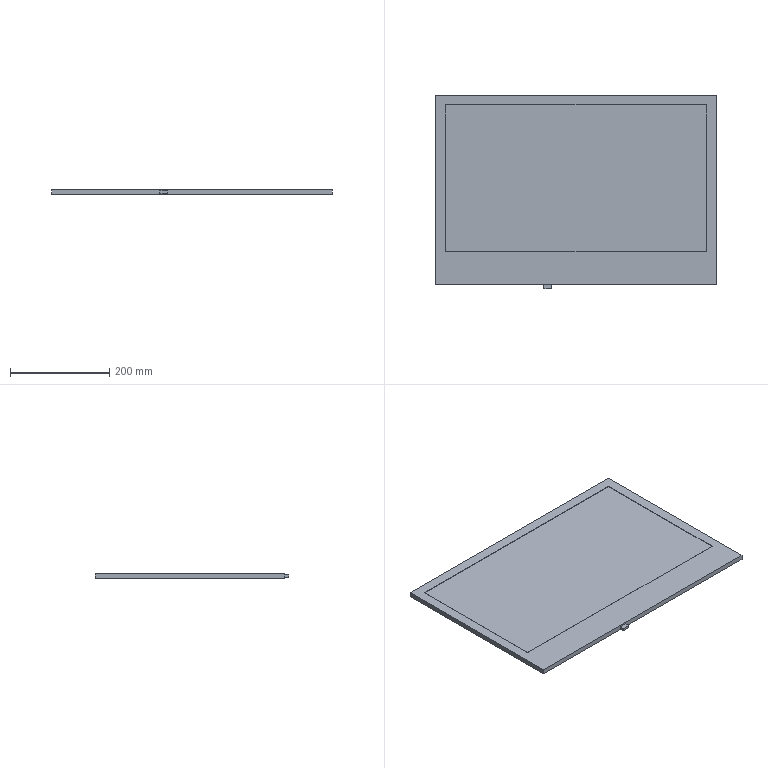Part | STEP file | 23.6 inch screen 01001 | 2 solids | 22 faces | box 564 x 390 x 10 mm | volume 1834790 mm3 | plane 22
STEP:
#1=CARTESIAN_POINT('',(0.,0.,0.));
#2=DIRECTION('',(0.,0.,1.));
#3=DIRECTION('',(1.,0.,0.));
#4=AXIS2_PLACEMENT_3D('',#1,#2,#3);
#5=CARTESIAN_POINT('',(282.,-190.,-5.));
#6=VERTEX_POINT('',#5);
#7=CARTESIAN_POINT('',(282.,190.,-5.));
#8=VERTEX_POINT('',#7);
#9=CARTESIAN_POINT('',(282.,-190.,-5.));
#10=DIRECTION('',(0.,1.,0.));
#11=VECTOR('',#10,1.);
#12=LINE('',#9,#11);
#13=CARTESIAN_POINT('',(0.,0.,-5.));
#14=DIRECTION('',(0.,0.,-1.));
#15=DIRECTION('',(-1.,0.,0.));
#16=AXIS2_PLACEMENT_3D('',#13,#14,#15);
#17=PLANE('',#16);
#18=CARTESIAN_POINT('',(-282.,-190.));
#19=DIRECTION('',(0.,1.));
#20=VECTOR('',#19,1.);
#21=LINE('',#18,#20);
#22=(GEOMETRIC_REPRESENTATION_CONTEXT(2)PARAMETRIC_REPRESENTATION_CONTEXT()REPRESENTATION_CONTEXT('',''));
#23=DEFINITIONAL_REPRESENTATION('',(#21),#22);
#24=PCURVE('',#17,#23);
#25=CARTESIAN_POINT('',(282.,-190.,5.));
#26=DIRECTION('',(-1.,0.,0.));
#27=DIRECTION('',(0.,0.,1.));
#28=AXIS2_PLACEMENT_3D('',#25,#26,#27);
#29=PLANE('',#28);
#30=CARTESIAN_POINT('',(-10.,0.));
#31=DIRECTION('',(0.,1.));
#32=VECTOR('',#31,1.);
#33=LINE('',#30,#32);
#34=(GEOMETRIC_REPRESENTATION_CONTEXT(2)PARAMETRIC_REPRESENTATION_CONTEXT()REPRESENTATION_CONTEXT('',''));
#35=DEFINITIONAL_REPRESENTATION('',(#33),#34);
#36=PCURVE('',#29,#35);
#37=SURFACE_CURVE('',#12,(#24,#36),.PCURVE_S1.);
#38=EDGE_CURVE('',#6,#8,#37,.T.);
#39=ORIENTED_EDGE('',*,*,#38,.F.);
#40=CARTESIAN_POINT('',(-282.,-190.,-5.));
#41=VERTEX_POINT('',#40);
#42=CARTESIAN_POINT('',(-282.,-190.,-5.));
#43=DIRECTION('',(1.,0.,0.));
#44=VECTOR('',#43,1.);
#45=LINE('',#42,#44);
#46=CARTESIAN_POINT('',(282.,-190.));
#47=DIRECTION('',(-1.,0.));
#48=VECTOR('',#47,1.);
#49=LINE('',#46,#48);
#50=(GEOMETRIC_REPRESENTATION_CONTEXT(2)PARAMETRIC_REPRESENTATION_CONTEXT()REPRESENTATION_CONTEXT('',''));
#51=DEFINITIONAL_REPRESENTATION('',(#49),#50);
#52=PCURVE('',#17,#51);
#53=CARTESIAN_POINT('',(-282.,-190.,5.));
#54=DIRECTION('',(0.,1.,0.));
#55=DIRECTION('',(0.,0.,1.));
#56=AXIS2_PLACEMENT_3D('',#53,#54,#55);
#57=PLANE('',#56);
#58=CARTESIAN_POINT('',(-10.,0.));
#59=DIRECTION('',(0.,1.));
#60=VECTOR('',#59,1.);
#61=LINE('',#58,#60);
#62=(GEOMETRIC_REPRESENTATION_CONTEXT(2)PARAMETRIC_REPRESENTATION_CONTEXT()REPRESENTATION_CONTEXT('',''));
#63=DEFINITIONAL_REPRESENTATION('',(#61),#62);
#64=PCURVE('',#57,#63);
#65=SURFACE_CURVE('',#45,(#52,#64),.PCURVE_S1.);
#66=EDGE_CURVE('',#41,#6,#65,.T.);
#67=ORIENTED_EDGE('',*,*,#66,.F.);
#68=CARTESIAN_POINT('',(-282.,190.,-5.));
#69=VERTEX_POINT('',#68);
#70=CARTESIAN_POINT('',(-282.,-190.,-5.));
#71=DIRECTION('',(0.,-1.,0.));
#72=VECTOR('',#71,1.);
#73=LINE('',#70,#72);
#74=CARTESIAN_POINT('',(282.,-190.));
#75=DIRECTION('',(0.,-1.));
#76=VECTOR('',#75,1.);
#77=LINE('',#74,#76);
#78=(GEOMETRIC_REPRESENTATION_CONTEXT(2)PARAMETRIC_REPRESENTATION_CONTEXT()REPRESENTATION_CONTEXT('',''));
#79=DEFINITIONAL_REPRESENTATION('',(#77),#78);
#80=PCURVE('',#17,#79);
#81=CARTESIAN_POINT('',(-282.,-190.,5.));
#82=DIRECTION('',(1.,0.,0.));
#83=DIRECTION('',(0.,0.,-1.));
#84=AXIS2_PLACEMENT_3D('',#81,#82,#83);
#85=PLANE('',#84);
#86=CARTESIAN_POINT('',(10.,0.));
#87=DIRECTION('',(0.,-1.));
#88=VECTOR('',#87,1.);
#89=LINE('',#86,#88);
#90=(GEOMETRIC_REPRESENTATION_CONTEXT(2)PARAMETRIC_REPRESENTATION_CONTEXT()REPRESENTATION_CONTEXT('',''));
#91=DEFINITIONAL_REPRESENTATION('',(#89),#90);
#92=PCURVE('',#85,#91);
#93=SURFACE_CURVE('',#73,(#80,#92),.PCURVE_S1.);
#94=EDGE_CURVE('',#69,#41,#93,.T.);
#95=ORIENTED_EDGE('',*,*,#94,.F.);
#96=CARTESIAN_POINT('',(-282.,190.,-5.));
#97=DIRECTION('',(-1.,0.,0.));
#98=VECTOR('',#97,1.);
#99=LINE('',#96,#98);
#100=CARTESIAN_POINT('',(282.,190.));
#101=DIRECTION('',(1.,0.));
#102=VECTOR('',#101,1.);
#103=LINE('',#100,#102);
#104=(GEOMETRIC_REPRESENTATION_CONTEXT(2)PARAMETRIC_REPRESENTATION_CONTEXT()REPRESENTATION_CONTEXT('',''));
#105=DEFINITIONAL_REPRESENTATION('',(#103),#104);
#106=PCURVE('',#17,#105);
#107=CARTESIAN_POINT('',(-282.,190.,5.));
#108=DIRECTION('',(0.,-1.,0.));
#109=DIRECTION('',(0.,0.,-1.));
#110=AXIS2_PLACEMENT_3D('',#107,#108,#109);
#111=PLANE('',#110);
#112=CARTESIAN_POINT('',(10.,0.));
#113=DIRECTION('',(0.,-1.));
#114=VECTOR('',#113,1.);
#115=LINE('',#112,#114);
#116=(GEOMETRIC_REPRESENTATION_CONTEXT(2)PARAMETRIC_REPRESENTATION_CONTEXT()REPRESENTATION_CONTEXT('',''));
#117=DEFINITIONAL_REPRESENTATION('',(#115),#116);
#118=PCURVE('',#111,#117);
#119=SURFACE_CURVE('',#99,(#106,#118),.PCURVE_S1.);
#120=EDGE_CURVE('',#8,#69,#119,.T.);
#121=ORIENTED_EDGE('',*,*,#120,.F.);
#122=EDGE_LOOP('',(#39,#67,#95,#121));
#123=FACE_BOUND('',#122,.T.);
#124=CARTESIAN_POINT('',(-262.,-125.,-5.));
#125=VERTEX_POINT('',#124);
#126=CARTESIAN_POINT('',(262.,-125.,-5.));
#127=VERTEX_POINT('',#126);
#128=CARTESIAN_POINT('',(-262.,-125.,-5.));
#129=DIRECTION('',(1.,0.,0.));
#130=VECTOR('',#129,1.);
#131=LINE('',#128,#130);
#132=CARTESIAN_POINT('',(262.,-125.));
#133=DIRECTION('',(-1.,0.));
#134=VECTOR('',#133,1.);
#135=LINE('',#132,#134);
#136=(GEOMETRIC_REPRESENTATION_CONTEXT(2)PARAMETRIC_REPRESENTATION_CONTEXT()REPRESENTATION_CONTEXT('',''));
#137=DEFINITIONAL_REPRESENTATION('',(#135),#136);
#138=PCURVE('',#17,#137);
#139=CARTESIAN_POINT('',(-262.,-125.,-4.));
#140=DIRECTION('',(0.,1.,0.));
#141=DIRECTION('',(0.,0.,1.));
#142=AXIS2_PLACEMENT_3D('',#139,#140,#141);
#143=PLANE('',#142);
#144=CARTESIAN_POINT('',(-1.,0.));
#145=DIRECTION('',(0.,1.));
#146=VECTOR('',#145,1.);
#147=LINE('',#144,#146);
#148=(GEOMETRIC_REPRESENTATION_CONTEXT(2)PARAMETRIC_REPRESENTATION_CONTEXT()REPRESENTATION_CONTEXT('',''));
#149=DEFINITIONAL_REPRESENTATION('',(#147),#148);
#150=PCURVE('',#143,#149);
#151=SURFACE_CURVE('',#131,(#138,#150),.PCURVE_S1.);
#152=EDGE_CURVE('',#125,#127,#151,.T.);
#153=ORIENTED_EDGE('',*,*,#152,.T.);
#154=CARTESIAN_POINT('',(262.,170.,-5.));
#155=VERTEX_POINT('',#154);
#156=CARTESIAN_POINT('',(262.,-125.,-5.));
#157=DIRECTION('',(0.,1.,0.));
#158=VECTOR('',#157,1.);
#159=LINE('',#156,#158);
#160=CARTESIAN_POINT('',(-262.,-125.));
#161=DIRECTION('',(0.,1.));
#162=VECTOR('',#161,1.);
#163=LINE('',#160,#162);
#164=(GEOMETRIC_REPRESENTATION_CONTEXT(2)PARAMETRIC_REPRESENTATION_CONTEXT()REPRESENTATION_CONTEXT('',''));
#165=DEFINITIONAL_REPRESENTATION('',(#163),#164);
#166=PCURVE('',#17,#165);
#167=CARTESIAN_POINT('',(262.,-125.,-4.));
#168=DIRECTION('',(-1.,0.,0.));
#169=DIRECTION('',(0.,0.,1.));
#170=AXIS2_PLACEMENT_3D('',#167,#168,#169);
#171=PLANE('',#170);
#172=CARTESIAN_POINT('',(-1.,0.));
#173=DIRECTION('',(0.,1.));
#174=VECTOR('',#173,1.);
#175=LINE('',#172,#174);
#176=(GEOMETRIC_REPRESENTATION_CONTEXT(2)PARAMETRIC_REPRESENTATION_CONTEXT()REPRESENTATION_CONTEXT('',''));
#177=DEFINITIONAL_REPRESENTATION('',(#175),#176);
#178=PCURVE('',#171,#177);
#179=SURFACE_CURVE('',#159,(#166,#178),.PCURVE_S1.);
#180=EDGE_CURVE('',#127,#155,#179,.T.);
#181=ORIENTED_EDGE('',*,*,#180,.T.);
#182=CARTESIAN_POINT('',(-262.,170.,-5.));
#183=VERTEX_POINT('',#182);
#184=CARTESIAN_POINT('',(-262.,170.,-5.));
#185=DIRECTION('',(-1.,0.,0.));
#186=VECTOR('',#185,1.);
#187=LINE('',#184,#186);
#188=CARTESIAN_POINT('',(262.,170.));
#189=DIRECTION('',(1.,0.));
#190=VECTOR('',#189,1.);
#191=LINE('',#188,#190);
#192=(GEOMETRIC_REPRESENTATION_CONTEXT(2)PARAMETRIC_REPRESENTATION_CONTEXT()REPRESENTATION_CONTEXT('',''));
#193=DEFINITIONAL_REPRESENTATION('',(#191),#192);
#194=PCURVE('',#17,#193);
#195=CARTESIAN_POINT('',(-262.,170.,-4.));
#196=DIRECTION('',(0.,-1.,0.));
#197=DIRECTION('',(0.,0.,-1.));
#198=AXIS2_PLACEMENT_3D('',#195,#196,#197);
#199=PLANE('',#198);
#200=CARTESIAN_POINT('',(1.,0.));
#201=DIRECTION('',(0.,-1.));
#202=VECTOR('',#201,1.);
#203=LINE('',#200,#202);
#204=(GEOMETRIC_REPRESENTATION_CONTEXT(2)PARAMETRIC_REPRESENTATION_CONTEXT()REPRESENTATION_CONTEXT('',''));
#205=DEFINITIONAL_REPRESENTATION('',(#203),#204);
#206=PCURVE('',#199,#205);
#207=SURFACE_CURVE('',#187,(#194,#206),.PCURVE_S1.);
#208=EDGE_CURVE('',#155,#183,#207,.T.);
#209=ORIENTED_EDGE('',*,*,#208,.T.);
#210=CARTESIAN_POINT('',(-262.,-125.,-5.));
#211=DIRECTION('',(0.,-1.,0.));
#212=VECTOR('',#211,1.);
#213=LINE('',#210,#212);
#214=CARTESIAN_POINT('',(262.,-125.));
#215=DIRECTION('',(0.,-1.));
#216=VECTOR('',#215,1.);
#217=LINE('',#214,#216);
#218=(GEOMETRIC_REPRESENTATION_CONTEXT(2)PARAMETRIC_REPRESENTATION_CONTEXT()REPRESENTATION_CONTEXT('',''));
#219=DEFINITIONAL_REPRESENTATION('',(#217),#218);
#220=PCURVE('',#17,#219);
#221=CARTESIAN_POINT('',(-262.,-125.,-4.));
#222=DIRECTION('',(1.,0.,0.));
#223=DIRECTION('',(0.,0.,-1.));
#224=AXIS2_PLACEMENT_3D('',#221,#222,#223);
#225=PLANE('',#224);
#226=CARTESIAN_POINT('',(1.,0.));
#227=DIRECTION('',(0.,-1.));
#228=VECTOR('',#227,1.);
#229=LINE('',#226,#228);
#230=(GEOMETRIC_REPRESENTATION_CONTEXT(2)PARAMETRIC_REPRESENTATION_CONTEXT()REPRESENTATION_CONTEXT('',''));
#231=DEFINITIONAL_REPRESENTATION('',(#229),#230);
#232=PCURVE('',#225,#231);
#233=SURFACE_CURVE('',#213,(#220,#232),.PCURVE_S1.);
#234=EDGE_CURVE('',#183,#125,#233,.T.);
#235=ORIENTED_EDGE('',*,*,#234,.T.);
#236=EDGE_LOOP('',(#153,#181,#209,#235));
#237=FACE_BOUND('',#236,.T.);
#238=ADVANCED_FACE('',(#123,#237),#17,.T.);
#239=ORIENTED_EDGE('',*,*,#38,.T.);
#240=CARTESIAN_POINT('',(282.,190.,5.));
#241=VERTEX_POINT('',#240);
#242=CARTESIAN_POINT('',(282.,190.,5.));
#243=DIRECTION('',(0.,0.,-1.));
#244=VECTOR('',#243,1.);
#245=LINE('',#242,#244);
#246=CARTESIAN_POINT('',(0.,380.));
#247=DIRECTION('',(-1.,0.));
#248=VECTOR('',#247,1.);
#249=LINE('',#246,#248);
#250=(GEOMETRIC_REPRESENTATION_CONTEXT(2)PARAMETRIC_REPRESENTATION_CONTEXT()REPRESENTATION_CONTEXT('',''));
#251=DEFINITIONAL_REPRESENTATION('',(#249),#250);
#252=PCURVE('',#29,#251);
#253=CARTESIAN_POINT('',(0.,564.));
#254=DIRECTION('',(1.,0.));
#255=VECTOR('',#254,1.);
#256=LINE('',#253,#255);
#257=(GEOMETRIC_REPRESENTATION_CONTEXT(2)PARAMETRIC_REPRESENTATION_CONTEXT()REPRESENTATION_CONTEXT('',''));
#258=DEFINITIONAL_REPRESENTATION('',(#256),#257);
#259=PCURVE('',#111,#258);
#260=SURFACE_CURVE('',#245,(#252,#259),.PCURVE_S1.);
#261=EDGE_CURVE('',#241,#8,#260,.T.);
#262=ORIENTED_EDGE('',*,*,#261,.F.);
#263=CARTESIAN_POINT('',(282.,-190.,5.));
#264=VERTEX_POINT('',#263);
#265=CARTESIAN_POINT('',(282.,-190.,5.));
#266=DIRECTION('',(0.,1.,0.));
#267=VECTOR('',#266,1.);
#268=LINE('',#265,#267);
#269=CARTESIAN_POINT('',(0.,0.));
#270=DIRECTION('',(0.,1.));
#271=VECTOR('',#270,1.);
#272=LINE('',#269,#271);
#273=(GEOMETRIC_REPRESENTATION_CONTEXT(2)PARAMETRIC_REPRESENTATION_CONTEXT()REPRESENTATION_CONTEXT('',''));
#274=DEFINITIONAL_REPRESENTATION('',(#272),#273);
#275=PCURVE('',#29,#274);
#276=CARTESIAN_POINT('',(0.,0.,5.));
#277=DIRECTION('',(0.,0.,-1.));
#278=DIRECTION('',(-1.,0.,0.));
#279=AXIS2_PLACEMENT_3D('',#276,#277,#278);
#280=PLANE('',#279);
#281=CARTESIAN_POINT('',(-282.,-190.));
#282=DIRECTION('',(0.,1.));
#283=VECTOR('',#282,1.);
#284=LINE('',#281,#283);
#285=(GEOMETRIC_REPRESENTATION_CONTEXT(2)PARAMETRIC_REPRESENTATION_CONTEXT()REPRESENTATION_CONTEXT('',''));
#286=DEFINITIONAL_REPRESENTATION('',(#284),#285);
#287=PCURVE('',#280,#286);
#288=SURFACE_CURVE('',#268,(#275,#287),.PCURVE_S1.);
#289=EDGE_CURVE('',#264,#241,#288,.T.);
#290=ORIENTED_EDGE('',*,*,#289,.F.);
#291=CARTESIAN_POINT('',(282.,-190.,5.));
#292=DIRECTION('',(0.,0.,-1.));
#293=VECTOR('',#292,1.);
#294=LINE('',#291,#293);
#295=CARTESIAN_POINT('',(0.,0.));
#296=DIRECTION('',(-1.,0.));
#297=VECTOR('',#296,1.);
#298=LINE('',#295,#297);
#299=(GEOMETRIC_REPRESENTATION_CONTEXT(2)PARAMETRIC_REPRESENTATION_CONTEXT()REPRESENTATION_CONTEXT('',''));
#300=DEFINITIONAL_REPRESENTATION('',(#298),#299);
#301=PCURVE('',#29,#300);
#302=CARTESIAN_POINT('',(0.,564.));
#303=DIRECTION('',(-1.,0.));
#304=VECTOR('',#303,1.);
#305=LINE('',#302,#304);
#306=(GEOMETRIC_REPRESENTATION_CONTEXT(2)PARAMETRIC_REPRESENTATION_CONTEXT()REPRESENTATION_CONTEXT('',''));
#307=DEFINITIONAL_REPRESENTATION('',(#305),#306);
#308=PCURVE('',#57,#307);
#309=SURFACE_CURVE('',#294,(#301,#308),.PCURVE_S1.);
#310=EDGE_CURVE('',#264,#6,#309,.T.);
#311=ORIENTED_EDGE('',*,*,#310,.T.);
#312=EDGE_LOOP('',(#239,#262,#290,#311));
#313=FACE_BOUND('',#312,.T.);
#314=ADVANCED_FACE('',(#313),#29,.F.);
#315=ORIENTED_EDGE('',*,*,#120,.T.);
#316=CARTESIAN_POINT('',(-282.,190.,5.));
#317=VERTEX_POINT('',#316);
#318=CARTESIAN_POINT('',(-282.,190.,5.));
#319=DIRECTION('',(0.,0.,-1.));
#320=VECTOR('',#319,1.);
#321=LINE('',#318,#320);
#322=CARTESIAN_POINT('',(0.,0.));
#323=DIRECTION('',(1.,0.));
#324=VECTOR('',#323,1.);
#325=LINE('',#322,#324);
#326=(GEOMETRIC_REPRESENTATION_CONTEXT(2)PARAMETRIC_REPRESENTATION_CONTEXT()REPRESENTATION_CONTEXT('',''));
#327=DEFINITIONAL_REPRESENTATION('',(#325),#326);
#328=PCURVE('',#111,#327);
#329=CARTESIAN_POINT('',(0.,380.));
#330=DIRECTION('',(1.,0.));
#331=VECTOR('',#330,1.);
#332=LINE('',#329,#331);
#333=(GEOMETRIC_REPRESENTATION_CONTEXT(2)PARAMETRIC_REPRESENTATION_CONTEXT()REPRESENTATION_CONTEXT('',''));
#334=DEFINITIONAL_REPRESENTATION('',(#332),#333);
#335=PCURVE('',#85,#334);
#336=SURFACE_CURVE('',#321,(#328,#335),.PCURVE_S1.);
#337=EDGE_CURVE('',#317,#69,#336,.T.);
#338=ORIENTED_EDGE('',*,*,#337,.F.);
#339=CARTESIAN_POINT('',(-282.,190.,5.));
#340=DIRECTION('',(-1.,0.,0.));
#341=VECTOR('',#340,1.);
#342=LINE('',#339,#341);
#343=CARTESIAN_POINT('',(0.,0.));
#344=DIRECTION('',(0.,-1.));
#345=VECTOR('',#344,1.);
#346=LINE('',#343,#345);
#347=(GEOMETRIC_REPRESENTATION_CONTEXT(2)PARAMETRIC_REPRESENTATION_CONTEXT()REPRESENTATION_CONTEXT('',''));
#348=DEFINITIONAL_REPRESENTATION('',(#346),#347);
#349=PCURVE('',#111,#348);
#350=CARTESIAN_POINT('',(282.,190.));
#351=DIRECTION('',(1.,0.));
#352=VECTOR('',#351,1.);
#353=LINE('',#350,#352);
#354=(GEOMETRIC_REPRESENTATION_CONTEXT(2)PARAMETRIC_REPRESENTATION_CONTEXT()REPRESENTATION_CONTEXT('',''));
#355=DEFINITIONAL_REPRESENTATION('',(#353),#354);
#356=PCURVE('',#280,#355);
#357=SURFACE_CURVE('',#342,(#349,#356),.PCURVE_S1.);
#358=EDGE_CURVE('',#241,#317,#357,.T.);
#359=ORIENTED_EDGE('',*,*,#358,.F.);
#360=ORIENTED_EDGE('',*,*,#261,.T.);
#361=EDGE_LOOP('',(#315,#338,#359,#360));
#362=FACE_BOUND('',#361,.T.);
#363=ADVANCED_FACE('',(#362),#111,.F.);
#364=ORIENTED_EDGE('',*,*,#94,.T.);
#365=CARTESIAN_POINT('',(-282.,-190.,5.));
#366=VERTEX_POINT('',#365);
#367=CARTESIAN_POINT('',(-282.,-190.,5.));
#368=DIRECTION('',(0.,0.,-1.));
#369=VECTOR('',#368,1.);
#370=LINE('',#367,#369);
#371=CARTESIAN_POINT('',(0.,0.));
#372=DIRECTION('',(1.,0.));
#373=VECTOR('',#372,1.);
#374=LINE('',#371,#373);
#375=(GEOMETRIC_REPRESENTATION_CONTEXT(2)PARAMETRIC_REPRESENTATION_CONTEXT()REPRESENTATION_CONTEXT('',''));
#376=DEFINITIONAL_REPRESENTATION('',(#374),#375);
#377=PCURVE('',#85,#376);
#378=CARTESIAN_POINT('',(0.,0.));
#379=DIRECTION('',(-1.,0.));
#380=VECTOR('',#379,1.);
#381=LINE('',#378,#380);
#382=(GEOMETRIC_REPRESENTATION_CONTEXT(2)PARAMETRIC_REPRESENTATION_CONTEXT()REPRESENTATION_CONTEXT('',''));
#383=DEFINITIONAL_REPRESENTATION('',(#381),#382);
#384=PCURVE('',#57,#383);
#385=SURFACE_CURVE('',#370,(#377,#384),.PCURVE_S1.);
#386=EDGE_CURVE('',#366,#41,#385,.T.);
#387=ORIENTED_EDGE('',*,*,#386,.F.);
#388=CARTESIAN_POINT('',(-282.,-190.,5.));
#389=DIRECTION('',(0.,-1.,0.));
#390=VECTOR('',#389,1.);
#391=LINE('',#388,#390);
#392=CARTESIAN_POINT('',(0.,0.));
#393=DIRECTION('',(0.,-1.));
#394=VECTOR('',#393,1.);
#395=LINE('',#392,#394);
#396=(GEOMETRIC_REPRESENTATION_CONTEXT(2)PARAMETRIC_REPRESENTATION_CONTEXT()REPRESENTATION_CONTEXT('',''));
#397=DEFINITIONAL_REPRESENTATION('',(#395),#396);
#398=PCURVE('',#85,#397);
#399=CARTESIAN_POINT('',(282.,-190.));
#400=DIRECTION('',(0.,-1.));
#401=VECTOR('',#400,1.);
#402=LINE('',#399,#401);
#403=(GEOMETRIC_REPRESENTATION_CONTEXT(2)PARAMETRIC_REPRESENTATION_CONTEXT()REPRESENTATION_CONTEXT('',''));
#404=DEFINITIONAL_REPRESENTATION('',(#402),#403);
#405=PCURVE('',#280,#404);
#406=SURFACE_CURVE('',#391,(#398,#405),.PCURVE_S1.);
#407=EDGE_CURVE('',#317,#366,#406,.T.);
#408=ORIENTED_EDGE('',*,*,#407,.F.);
#409=ORIENTED_EDGE('',*,*,#337,.T.);
#410=EDGE_LOOP('',(#364,#387,#408,#409));
#411=FACE_BOUND('',#410,.T.);
#412=ADVANCED_FACE('',(#411),#85,.F.);
#413=ORIENTED_EDGE('',*,*,#66,.T.);
#414=ORIENTED_EDGE('',*,*,#310,.F.);
#415=CARTESIAN_POINT('',(-282.,-190.,5.));
#416=DIRECTION('',(1.,0.,0.));
#417=VECTOR('',#416,1.);
#418=LINE('',#415,#417);
#419=CARTESIAN_POINT('',(0.,0.));
#420=DIRECTION('',(0.,1.));
#421=VECTOR('',#420,1.);
#422=LINE('',#419,#421);
#423=(GEOMETRIC_REPRESENTATION_CONTEXT(2)PARAMETRIC_REPRESENTATION_CONTEXT()REPRESENTATION_CONTEXT('',''));
#424=DEFINITIONAL_REPRESENTATION('',(#422),#423);
#425=PCURVE('',#57,#424);
#426=CARTESIAN_POINT('',(282.,-190.));
#427=DIRECTION('',(-1.,0.));
#428=VECTOR('',#427,1.);
#429=LINE('',#426,#428);
#430=(GEOMETRIC_REPRESENTATION_CONTEXT(2)PARAMETRIC_REPRESENTATION_CONTEXT()REPRESENTATION_CONTEXT('',''));
#431=DEFINITIONAL_REPRESENTATION('',(#429),#430);
#432=PCURVE('',#280,#431);
#433=SURFACE_CURVE('',#418,(#425,#432),.PCURVE_S1.);
#434=EDGE_CURVE('',#366,#264,#433,.T.);
#435=ORIENTED_EDGE('',*,*,#434,.F.);
#436=ORIENTED_EDGE('',*,*,#386,.T.);
#437=EDGE_LOOP('',(#413,#414,#435,#436));
#438=FACE_BOUND('',#437,.T.);
#439=ADVANCED_FACE('',(#438),#57,.F.);
#440=CARTESIAN_POINT('',(262.,170.,5.));
#441=VERTEX_POINT('',#440);
#442=CARTESIAN_POINT('',(-262.,170.,5.));
#443=VERTEX_POINT('',#442);
#444=CARTESIAN_POINT('',(-262.,170.,5.));
#445=DIRECTION('',(-1.,0.,0.));
#446=VECTOR('',#445,1.);
#447=LINE('',#444,#446);
#448=CARTESIAN_POINT('',(262.,170.));
#449=DIRECTION('',(1.,0.));
#450=VECTOR('',#449,1.);
#451=LINE('',#448,#450);
#452=(GEOMETRIC_REPRESENTATION_CONTEXT(2)PARAMETRIC_REPRESENTATION_CONTEXT()REPRESENTATION_CONTEXT('',''));
#453=DEFINITIONAL_REPRESENTATION('',(#451),#452);
#454=PCURVE('',#280,#453);
#455=CARTESIAN_POINT('',(-262.,170.,4.));
#456=DIRECTION('',(0.,1.,0.));
#457=DIRECTION('',(0.,0.,1.));
#458=AXIS2_PLACEMENT_3D('',#455,#456,#457);
#459=PLANE('',#458);
#460=CARTESIAN_POINT('',(1.,0.));
#461=DIRECTION('',(0.,-1.));
#462=VECTOR('',#461,1.);
#463=LINE('',#460,#462);
#464=(GEOMETRIC_REPRESENTATION_CONTEXT(2)PARAMETRIC_REPRESENTATION_CONTEXT()REPRESENTATION_CONTEXT('',''));
#465=DEFINITIONAL_REPRESENTATION('',(#463),#464);
#466=PCURVE('',#459,#465);
#467=SURFACE_CURVE('',#447,(#454,#466),.PCURVE_S1.);
#468=EDGE_CURVE('',#441,#443,#467,.T.);
#469=ORIENTED_EDGE('',*,*,#468,.F.);
#470=CARTESIAN_POINT('',(262.,-125.,5.));
#471=VERTEX_POINT('',#470);
#472=CARTESIAN_POINT('',(262.,-125.,5.));
#473=DIRECTION('',(0.,1.,0.));
#474=VECTOR('',#473,1.);
#475=LINE('',#472,#474);
#476=CARTESIAN_POINT('',(-262.,-125.));
#477=DIRECTION('',(0.,1.));
#478=VECTOR('',#477,1.);
#479=LINE('',#476,#478);
#480=(GEOMETRIC_REPRESENTATION_CONTEXT(2)PARAMETRIC_REPRESENTATION_CONTEXT()REPRESENTATION_CONTEXT('',''));
#481=DEFINITIONAL_REPRESENTATION('',(#479),#480);
#482=PCURVE('',#280,#481);
#483=CARTESIAN_POINT('',(262.,-125.,4.));
#484=DIRECTION('',(1.,0.,0.));
#485=DIRECTION('',(0.,0.,-1.));
#486=AXIS2_PLACEMENT_3D('',#483,#484,#485);
#487=PLANE('',#486);
#488=CARTESIAN_POINT('',(-1.,0.));
#489=DIRECTION('',(0.,1.));
#490=VECTOR('',#489,1.);
#491=LINE('',#488,#490);
#492=(GEOMETRIC_REPRESENTATION_CONTEXT(2)PARAMETRIC_REPRESENTATION_CONTEXT()REPRESENTATION_CONTEXT('',''));
#493=DEFINITIONAL_REPRESENTATION('',(#491),#492);
#494=PCURVE('',#487,#493);
#495=SURFACE_CURVE('',#475,(#482,#494),.PCURVE_S1.);
#496=EDGE_CURVE('',#471,#441,#495,.T.);
#497=ORIENTED_EDGE('',*,*,#496,.F.);
#498=CARTESIAN_POINT('',(-262.,-125.,5.));
#499=VERTEX_POINT('',#498);
#500=CARTESIAN_POINT('',(-262.,-125.,5.));
#501=DIRECTION('',(1.,0.,0.));
#502=VECTOR('',#501,1.);
#503=LINE('',#500,#502);
#504=CARTESIAN_POINT('',(262.,-125.));
#505=DIRECTION('',(-1.,0.));
#506=VECTOR('',#505,1.);
#507=LINE('',#504,#506);
#508=(GEOMETRIC_REPRESENTATION_CONTEXT(2)PARAMETRIC_REPRESENTATION_CONTEXT()REPRESENTATION_CONTEXT('',''));
#509=DEFINITIONAL_REPRESENTATION('',(#507),#508);
#510=PCURVE('',#280,#509);
#511=CARTESIAN_POINT('',(-262.,-125.,4.));
#512=DIRECTION('',(0.,-1.,0.));
#513=DIRECTION('',(0.,0.,-1.));
#514=AXIS2_PLACEMENT_3D('',#511,#512,#513);
#515=PLANE('',#514);
#516=CARTESIAN_POINT('',(-1.,0.));
#517=DIRECTION('',(0.,1.));
#518=VECTOR('',#517,1.);
#519=LINE('',#516,#518);
#520=(GEOMETRIC_REPRESENTATION_CONTEXT(2)PARAMETRIC_REPRESENTATION_CONTEXT()REPRESENTATION_CONTEXT('',''));
#521=DEFINITIONAL_REPRESENTATION('',(#519),#520);
#522=PCURVE('',#515,#521);
#523=SURFACE_CURVE('',#503,(#510,#522),.PCURVE_S1.);
#524=EDGE_CURVE('',#499,#471,#523,.T.);
#525=ORIENTED_EDGE('',*,*,#524,.F.);
#526=CARTESIAN_POINT('',(-262.,-125.,5.));
#527=DIRECTION('',(0.,-1.,0.));
#528=VECTOR('',#527,1.);
#529=LINE('',#526,#528);
#530=CARTESIAN_POINT('',(262.,-125.));
#531=DIRECTION('',(0.,-1.));
#532=VECTOR('',#531,1.);
#533=LINE('',#530,#532);
#534=(GEOMETRIC_REPRESENTATION_CONTEXT(2)PARAMETRIC_REPRESENTATION_CONTEXT()REPRESENTATION_CONTEXT('',''));
#535=DEFINITIONAL_REPRESENTATION('',(#533),#534);
#536=PCURVE('',#280,#535);
#537=CARTESIAN_POINT('',(-262.,-125.,4.));
#538=DIRECTION('',(-1.,0.,0.));
#539=DIRECTION('',(0.,0.,1.));
#540=AXIS2_PLACEMENT_3D('',#537,#538,#539);
#541=PLANE('',#540);
#542=CARTESIAN_POINT('',(1.,0.));
#543=DIRECTION('',(0.,-1.));
#544=VECTOR('',#543,1.);
#545=LINE('',#542,#544);
#546=(GEOMETRIC_REPRESENTATION_CONTEXT(2)PARAMETRIC_REPRESENTATION_CONTEXT()REPRESENTATION_CONTEXT('',''));
#547=DEFINITIONAL_REPRESENTATION('',(#545),#546);
#548=PCURVE('',#541,#547);
#549=SURFACE_CURVE('',#529,(#536,#548),.PCURVE_S1.);
#550=EDGE_CURVE('',#443,#499,#549,.T.);
#551=ORIENTED_EDGE('',*,*,#550,.F.);
#552=EDGE_LOOP('',(#469,#497,#525,#551));
#553=FACE_BOUND('',#552,.T.);
#554=ORIENTED_EDGE('',*,*,#289,.T.);
#555=ORIENTED_EDGE('',*,*,#358,.T.);
#556=ORIENTED_EDGE('',*,*,#407,.T.);
#557=ORIENTED_EDGE('',*,*,#434,.T.);
#558=EDGE_LOOP('',(#554,#555,#556,#557));
#559=FACE_BOUND('',#558,.T.);
#560=ADVANCED_FACE('',(#553,#559),#280,.F.);
#561=ORIENTED_EDGE('',*,*,#496,.T.);
#562=CARTESIAN_POINT('',(262.,170.,4.));
#563=VERTEX_POINT('',#562);
#564=CARTESIAN_POINT('',(262.,170.,4.));
#565=DIRECTION('',(0.,0.,1.));
#566=VECTOR('',#565,1.);
#567=LINE('',#564,#566);
#568=CARTESIAN_POINT('',(0.,295.));
#569=DIRECTION('',(-1.,0.));
#570=VECTOR('',#569,1.);
#571=LINE('',#568,#570);
#572=(GEOMETRIC_REPRESENTATION_CONTEXT(2)PARAMETRIC_REPRESENTATION_CONTEXT()REPRESENTATION_CONTEXT('',''));
#573=DEFINITIONAL_REPRESENTATION('',(#571),#572);
#574=PCURVE('',#487,#573);
#575=CARTESIAN_POINT('',(0.,524.));
#576=DIRECTION('',(1.,0.));
#577=VECTOR('',#576,1.);
#578=LINE('',#575,#577);
#579=(GEOMETRIC_REPRESENTATION_CONTEXT(2)PARAMETRIC_REPRESENTATION_CONTEXT()REPRESENTATION_CONTEXT('',''));
#580=DEFINITIONAL_REPRESENTATION('',(#578),#579);
#581=PCURVE('',#459,#580);
#582=SURFACE_CURVE('',#567,(#574,#581),.PCURVE_S1.);
#583=EDGE_CURVE('',#563,#441,#582,.T.);
#584=ORIENTED_EDGE('',*,*,#583,.F.);
#585=CARTESIAN_POINT('',(262.,-125.,4.));
#586=VERTEX_POINT('',#585);
#587=CARTESIAN_POINT('',(262.,-125.,4.));
#588=DIRECTION('',(0.,1.,0.));
#589=VECTOR('',#588,1.);
#590=LINE('',#587,#589);
#591=CARTESIAN_POINT('',(0.,0.));
#592=DIRECTION('',(0.,1.));
#593=VECTOR('',#592,1.);
#594=LINE('',#591,#593);
#595=(GEOMETRIC_REPRESENTATION_CONTEXT(2)PARAMETRIC_REPRESENTATION_CONTEXT()REPRESENTATION_CONTEXT('',''));
#596=DEFINITIONAL_REPRESENTATION('',(#594),#595);
#597=PCURVE('',#487,#596);
#598=CARTESIAN_POINT('',(0.,0.,4.));
#599=DIRECTION('',(0.,0.,-1.));
#600=DIRECTION('',(-1.,0.,0.));
#601=AXIS2_PLACEMENT_3D('',#598,#599,#600);
#602=PLANE('',#601);
#603=CARTESIAN_POINT('',(-262.,-125.));
#604=DIRECTION('',(0.,1.));
#605=VECTOR('',#604,1.);
#606=LINE('',#603,#605);
#607=(GEOMETRIC_REPRESENTATION_CONTEXT(2)PARAMETRIC_REPRESENTATION_CONTEXT()REPRESENTATION_CONTEXT('',''));
#608=DEFINITIONAL_REPRESENTATION('',(#606),#607);
#609=PCURVE('',#602,#608);
#610=SURFACE_CURVE('',#590,(#597,#609),.PCURVE_S1.);
#611=EDGE_CURVE('',#586,#563,#610,.T.);
#612=ORIENTED_EDGE('',*,*,#611,.F.);
#613=CARTESIAN_POINT('',(262.,-125.,4.));
#614=DIRECTION('',(0.,0.,1.));
#615=VECTOR('',#614,1.);
#616=LINE('',#613,#615);
#617=CARTESIAN_POINT('',(0.,0.));
#618=DIRECTION('',(-1.,0.));
#619=VECTOR('',#618,1.);
#620=LINE('',#617,#619);
#621=(GEOMETRIC_REPRESENTATION_CONTEXT(2)PARAMETRIC_REPRESENTATION_CONTEXT()REPRESENTATION_CONTEXT('',''));
#622=DEFINITIONAL_REPRESENTATION('',(#620),#621);
#623=PCURVE('',#487,#622);
#624=CARTESIAN_POINT('',(0.,524.));
#625=DIRECTION('',(-1.,0.));
#626=VECTOR('',#625,1.);
#627=LINE('',#624,#626);
#628=(GEOMETRIC_REPRESENTATION_CONTEXT(2)PARAMETRIC_REPRESENTATION_CONTEXT()REPRESENTATION_CONTEXT('',''));
#629=DEFINITIONAL_REPRESENTATION('',(#627),#628);
#630=PCURVE('',#515,#629);
#631=SURFACE_CURVE('',#616,(#623,#630),.PCURVE_S1.);
#632=EDGE_CURVE('',#586,#471,#631,.T.);
#633=ORIENTED_EDGE('',*,*,#632,.T.);
#634=EDGE_LOOP('',(#561,#584,#612,#633));
#635=FACE_BOUND('',#634,.T.);
#636=ADVANCED_FACE('',(#635),#487,.F.);
#637=ORIENTED_EDGE('',*,*,#524,.T.);
#638=ORIENTED_EDGE('',*,*,#632,.F.);
#639=CARTESIAN_POINT('',(-262.,-125.,4.));
#640=VERTEX_POINT('',#639);
#641=CARTESIAN_POINT('',(-262.,-125.,4.));
#642=DIRECTION('',(1.,0.,0.));
#643=VECTOR('',#642,1.);
#644=LINE('',#641,#643);
#645=CARTESIAN_POINT('',(0.,0.));
#646=DIRECTION('',(0.,1.));
#647=VECTOR('',#646,1.);
#648=LINE('',#645,#647);
#649=(GEOMETRIC_REPRESENTATION_CONTEXT(2)PARAMETRIC_REPRESENTATION_CONTEXT()REPRESENTATION_CONTEXT('',''));
#650=DEFINITIONAL_REPRESENTATION('',(#648),#649);
#651=PCURVE('',#515,#650);
#652=CARTESIAN_POINT('',(262.,-125.));
#653=DIRECTION('',(-1.,0.));
#654=VECTOR('',#653,1.);
#655=LINE('',#652,#654);
#656=(GEOMETRIC_REPRESENTATION_CONTEXT(2)PARAMETRIC_REPRESENTATION_CONTEXT()REPRESENTATION_CONTEXT('',''));
#657=DEFINITIONAL_REPRESENTATION('',(#655),#656);
#658=PCURVE('',#602,#657);
#659=SURFACE_CURVE('',#644,(#651,#658),.PCURVE_S1.);
#660=EDGE_CURVE('',#640,#586,#659,.T.);
#661=ORIENTED_EDGE('',*,*,#660,.F.);
#662=CARTESIAN_POINT('',(-262.,-125.,4.));
#663=DIRECTION('',(0.,0.,1.));
#664=VECTOR('',#663,1.);
#665=LINE('',#662,#664);
#666=CARTESIAN_POINT('',(0.,0.));
#667=DIRECTION('',(-1.,0.));
#668=VECTOR('',#667,1.);
#669=LINE('',#666,#668);
#670=(GEOMETRIC_REPRESENTATION_CONTEXT(2)PARAMETRIC_REPRESENTATION_CONTEXT()REPRESENTATION_CONTEXT('',''));
#671=DEFINITIONAL_REPRESENTATION('',(#669),#670);
#672=PCURVE('',#515,#671);
#673=CARTESIAN_POINT('',(0.,0.));
#674=DIRECTION('',(1.,0.));
#675=VECTOR('',#674,1.);
#676=LINE('',#673,#675);
#677=(GEOMETRIC_REPRESENTATION_CONTEXT(2)PARAMETRIC_REPRESENTATION_CONTEXT()REPRESENTATION_CONTEXT('',''));
#678=DEFINITIONAL_REPRESENTATION('',(#676),#677);
#679=PCURVE('',#541,#678);
#680=SURFACE_CURVE('',#665,(#672,#679),.PCURVE_S1.);
#681=EDGE_CURVE('',#640,#499,#680,.T.);
#682=ORIENTED_EDGE('',*,*,#681,.T.);
#683=EDGE_LOOP('',(#637,#638,#661,#682));
#684=FACE_BOUND('',#683,.T.);
#685=ADVANCED_FACE('',(#684),#515,.F.);
#686=ORIENTED_EDGE('',*,*,#550,.T.);
#687=ORIENTED_EDGE('',*,*,#681,.F.);
#688=CARTESIAN_POINT('',(-262.,170.,4.));
#689=VERTEX_POINT('',#688);
#690=CARTESIAN_POINT('',(-262.,-125.,4.));
#691=DIRECTION('',(0.,-1.,0.));
#692=VECTOR('',#691,1.);
#693=LINE('',#690,#692);
#694=CARTESIAN_POINT('',(0.,0.));
#695=DIRECTION('',(0.,-1.));
#696=VECTOR('',#695,1.);
#697=LINE('',#694,#696);
#698=(GEOMETRIC_REPRESENTATION_CONTEXT(2)PARAMETRIC_REPRESENTATION_CONTEXT()REPRESENTATION_CONTEXT('',''));
#699=DEFINITIONAL_REPRESENTATION('',(#697),#698);
#700=PCURVE('',#541,#699);
#701=CARTESIAN_POINT('',(262.,-125.));
#702=DIRECTION('',(0.,-1.));
#703=VECTOR('',#702,1.);
#704=LINE('',#701,#703);
#705=(GEOMETRIC_REPRESENTATION_CONTEXT(2)PARAMETRIC_REPRESENTATION_CONTEXT()REPRESENTATION_CONTEXT('',''));
#706=DEFINITIONAL_REPRESENTATION('',(#704),#705);
#707=PCURVE('',#602,#706);
#708=SURFACE_CURVE('',#693,(#700,#707),.PCURVE_S1.);
#709=EDGE_CURVE('',#689,#640,#708,.T.);
#710=ORIENTED_EDGE('',*,*,#709,.F.);
#711=CARTESIAN_POINT('',(-262.,170.,4.));
#712=DIRECTION('',(0.,0.,1.));
#713=VECTOR('',#712,1.);
#714=LINE('',#711,#713);
#715=CARTESIAN_POINT('',(0.,295.));
#716=DIRECTION('',(1.,0.));
#717=VECTOR('',#716,1.);
#718=LINE('',#715,#717);
#719=(GEOMETRIC_REPRESENTATION_CONTEXT(2)PARAMETRIC_REPRESENTATION_CONTEXT()REPRESENTATION_CONTEXT('',''));
#720=DEFINITIONAL_REPRESENTATION('',(#718),#719);
#721=PCURVE('',#541,#720);
#722=CARTESIAN_POINT('',(0.,0.));
#723=DIRECTION('',(1.,0.));
#724=VECTOR('',#723,1.);
#725=LINE('',#722,#724);
#726=(GEOMETRIC_REPRESENTATION_CONTEXT(2)PARAMETRIC_REPRESENTATION_CONTEXT()REPRESENTATION_CONTEXT('',''));
#727=DEFINITIONAL_REPRESENTATION('',(#725),#726);
#728=PCURVE('',#459,#727);
#729=SURFACE_CURVE('',#714,(#721,#728),.PCURVE_S1.);
#730=EDGE_CURVE('',#689,#443,#729,.T.);
#731=ORIENTED_EDGE('',*,*,#730,.T.);
#732=EDGE_LOOP('',(#686,#687,#710,#731));
#733=FACE_BOUND('',#732,.T.);
#734=ADVANCED_FACE('',(#733),#541,.F.);
#735=ORIENTED_EDGE('',*,*,#468,.T.);
#736=ORIENTED_EDGE('',*,*,#730,.F.);
#737=CARTESIAN_POINT('',(-262.,170.,4.));
#738=DIRECTION('',(-1.,0.,0.));
#739=VECTOR('',#738,1.);
#740=LINE('',#737,#739);
#741=CARTESIAN_POINT('',(0.,0.));
#742=DIRECTION('',(0.,-1.));
#743=VECTOR('',#742,1.);
#744=LINE('',#741,#743);
#745=(GEOMETRIC_REPRESENTATION_CONTEXT(2)PARAMETRIC_REPRESENTATION_CONTEXT()REPRESENTATION_CONTEXT('',''));
#746=DEFINITIONAL_REPRESENTATION('',(#744),#745);
#747=PCURVE('',#459,#746);
#748=CARTESIAN_POINT('',(262.,170.));
#749=DIRECTION('',(1.,0.));
#750=VECTOR('',#749,1.);
#751=LINE('',#748,#750);
#752=(GEOMETRIC_REPRESENTATION_CONTEXT(2)PARAMETRIC_REPRESENTATION_CONTEXT()REPRESENTATION_CONTEXT('',''));
#753=DEFINITIONAL_REPRESENTATION('',(#751),#752);
#754=PCURVE('',#602,#753);
#755=SURFACE_CURVE('',#740,(#747,#754),.PCURVE_S1.);
#756=EDGE_CURVE('',#563,#689,#755,.T.);
#757=ORIENTED_EDGE('',*,*,#756,.F.);
#758=ORIENTED_EDGE('',*,*,#583,.T.);
#759=EDGE_LOOP('',(#735,#736,#757,#758));
#760=FACE_BOUND('',#759,.T.);
#761=ADVANCED_FACE('',(#760),#459,.F.);
#762=ORIENTED_EDGE('',*,*,#611,.T.);
#763=ORIENTED_EDGE('',*,*,#756,.T.);
#764=ORIENTED_EDGE('',*,*,#709,.T.);
#765=ORIENTED_EDGE('',*,*,#660,.T.);
#766=EDGE_LOOP('',(#762,#763,#764,#765));
#767=FACE_BOUND('',#766,.T.);
#768=ADVANCED_FACE('',(#767),#602,.F.);
#769=ORIENTED_EDGE('',*,*,#180,.F.);
#770=CARTESIAN_POINT('',(262.,-125.,-4.));
#771=VERTEX_POINT('',#770);
#772=CARTESIAN_POINT('',(262.,-125.,-4.));
#773=DIRECTION('',(0.,0.,-1.));
#774=VECTOR('',#773,1.);
#775=LINE('',#772,#774);
#776=CARTESIAN_POINT('',(0.,0.));
#777=DIRECTION('',(-1.,0.));
#778=VECTOR('',#777,1.);
#779=LINE('',#776,#778);
#780=(GEOMETRIC_REPRESENTATION_CONTEXT(2)PARAMETRIC_REPRESENTATION_CONTEXT()REPRESENTATION_CONTEXT('',''));
#781=DEFINITIONAL_REPRESENTATION('',(#779),#780);
#782=PCURVE('',#171,#781);
#783=CARTESIAN_POINT('',(0.,524.));
#784=DIRECTION('',(-1.,0.));
#785=VECTOR('',#784,1.);
#786=LINE('',#783,#785);
#787=(GEOMETRIC_REPRESENTATION_CONTEXT(2)PARAMETRIC_REPRESENTATION_CONTEXT()REPRESENTATION_CONTEXT('',''));
#788=DEFINITIONAL_REPRESENTATION('',(#786),#787);
#789=PCURVE('',#143,#788);
#790=SURFACE_CURVE('',#775,(#782,#789),.PCURVE_S1.);
#791=EDGE_CURVE('',#771,#127,#790,.T.);
#792=ORIENTED_EDGE('',*,*,#791,.F.);
#793=CARTESIAN_POINT('',(262.,170.,-4.));
#794=VERTEX_POINT('',#793);
#795=CARTESIAN_POINT('',(262.,-125.,-4.));
#796=DIRECTION('',(0.,1.,0.));
#797=VECTOR('',#796,1.);
#798=LINE('',#795,#797);
#799=CARTESIAN_POINT('',(0.,0.));
#800=DIRECTION('',(0.,1.));
#801=VECTOR('',#800,1.);
#802=LINE('',#799,#801);
#803=(GEOMETRIC_REPRESENTATION_CONTEXT(2)PARAMETRIC_REPRESENTATION_CONTEXT()REPRESENTATION_CONTEXT('',''));
#804=DEFINITIONAL_REPRESENTATION('',(#802),#803);
#805=PCURVE('',#171,#804);
#806=CARTESIAN_POINT('',(0.,0.,-4.));
#807=DIRECTION('',(0.,0.,1.));
#808=DIRECTION('',(-1.,0.,0.));
#809=AXIS2_PLACEMENT_3D('',#806,#807,#808);
#810=PLANE('',#809);
#811=CARTESIAN_POINT('',(-262.,125.));
#812=DIRECTION('',(0.,-1.));
#813=VECTOR('',#812,1.);
#814=LINE('',#811,#813);
#815=(GEOMETRIC_REPRESENTATION_CONTEXT(2)PARAMETRIC_REPRESENTATION_CONTEXT()REPRESENTATION_CONTEXT('',''));
#816=DEFINITIONAL_REPRESENTATION('',(#814),#815);
#817=PCURVE('',#810,#816);
#818=SURFACE_CURVE('',#798,(#805,#817),.PCURVE_S1.);
#819=EDGE_CURVE('',#771,#794,#818,.T.);
#820=ORIENTED_EDGE('',*,*,#819,.T.);
#821=CARTESIAN_POINT('',(262.,170.,-4.));
#822=DIRECTION('',(0.,0.,-1.));
#823=VECTOR('',#822,1.);
#824=LINE('',#821,#823);
#825=CARTESIAN_POINT('',(0.,295.));
#826=DIRECTION('',(-1.,0.));
#827=VECTOR('',#826,1.);
#828=LINE('',#825,#827);
#829=(GEOMETRIC_REPRESENTATION_CONTEXT(2)PARAMETRIC_REPRESENTATION_CONTEXT()REPRESENTATION_CONTEXT('',''));
#830=DEFINITIONAL_REPRESENTATION('',(#828),#829);
#831=PCURVE('',#171,#830);
#832=CARTESIAN_POINT('',(0.,524.));
#833=DIRECTION('',(1.,0.));
#834=VECTOR('',#833,1.);
#835=LINE('',#832,#834);
#836=(GEOMETRIC_REPRESENTATION_CONTEXT(2)PARAMETRIC_REPRESENTATION_CONTEXT()REPRESENTATION_CONTEXT('',''));
#837=DEFINITIONAL_REPRESENTATION('',(#835),#836);
#838=PCURVE('',#199,#837);
#839=SURFACE_CURVE('',#824,(#831,#838),.PCURVE_S1.);
#840=EDGE_CURVE('',#794,#155,#839,.T.);
#841=ORIENTED_EDGE('',*,*,#840,.T.);
#842=EDGE_LOOP('',(#769,#792,#820,#841));
#843=FACE_BOUND('',#842,.T.);
#844=ADVANCED_FACE('',(#843),#171,.T.);
#845=ORIENTED_EDGE('',*,*,#208,.F.);
#846=ORIENTED_EDGE('',*,*,#840,.F.);
#847=CARTESIAN_POINT('',(-262.,170.,-4.));
#848=VERTEX_POINT('',#847);
#849=CARTESIAN_POINT('',(-262.,170.,-4.));
#850=DIRECTION('',(-1.,0.,0.));
#851=VECTOR('',#850,1.);
#852=LINE('',#849,#851);
#853=CARTESIAN_POINT('',(0.,0.));
#854=DIRECTION('',(0.,-1.));
#855=VECTOR('',#854,1.);
#856=LINE('',#853,#855);
#857=(GEOMETRIC_REPRESENTATION_CONTEXT(2)PARAMETRIC_REPRESENTATION_CONTEXT()REPRESENTATION_CONTEXT('',''));
#858=DEFINITIONAL_REPRESENTATION('',(#856),#857);
#859=PCURVE('',#199,#858);
#860=CARTESIAN_POINT('',(262.,-170.));
#861=DIRECTION('',(1.,0.));
#862=VECTOR('',#861,1.);
#863=LINE('',#860,#862);
#864=(GEOMETRIC_REPRESENTATION_CONTEXT(2)PARAMETRIC_REPRESENTATION_CONTEXT()REPRESENTATION_CONTEXT('',''));
#865=DEFINITIONAL_REPRESENTATION('',(#863),#864);
#866=PCURVE('',#810,#865);
#867=SURFACE_CURVE('',#852,(#859,#866),.PCURVE_S1.);
#868=EDGE_CURVE('',#794,#848,#867,.T.);
#869=ORIENTED_EDGE('',*,*,#868,.T.);
#870=CARTESIAN_POINT('',(-262.,170.,-4.));
#871=DIRECTION('',(0.,0.,-1.));
#872=VECTOR('',#871,1.);
#873=LINE('',#870,#872);
#874=CARTESIAN_POINT('',(0.,0.));
#875=DIRECTION('',(1.,0.));
#876=VECTOR('',#875,1.);
#877=LINE('',#874,#876);
#878=(GEOMETRIC_REPRESENTATION_CONTEXT(2)PARAMETRIC_REPRESENTATION_CONTEXT()REPRESENTATION_CONTEXT('',''));
#879=DEFINITIONAL_REPRESENTATION('',(#877),#878);
#880=PCURVE('',#199,#879);
#881=CARTESIAN_POINT('',(0.,295.));
#882=DIRECTION('',(1.,0.));
#883=VECTOR('',#882,1.);
#884=LINE('',#881,#883);
#885=(GEOMETRIC_REPRESENTATION_CONTEXT(2)PARAMETRIC_REPRESENTATION_CONTEXT()REPRESENTATION_CONTEXT('',''));
#886=DEFINITIONAL_REPRESENTATION('',(#884),#885);
#887=PCURVE('',#225,#886);
#888=SURFACE_CURVE('',#873,(#880,#887),.PCURVE_S1.);
#889=EDGE_CURVE('',#848,#183,#888,.T.);
#890=ORIENTED_EDGE('',*,*,#889,.T.);
#891=EDGE_LOOP('',(#845,#846,#869,#890));
#892=FACE_BOUND('',#891,.T.);
#893=ADVANCED_FACE('',(#892),#199,.T.);
#894=ORIENTED_EDGE('',*,*,#234,.F.);
#895=ORIENTED_EDGE('',*,*,#889,.F.);
#896=CARTESIAN_POINT('',(-262.,-125.,-4.));
#897=VERTEX_POINT('',#896);
#898=CARTESIAN_POINT('',(-262.,-125.,-4.));
#899=DIRECTION('',(0.,-1.,0.));
#900=VECTOR('',#899,1.);
#901=LINE('',#898,#900);
#902=CARTESIAN_POINT('',(0.,0.));
#903=DIRECTION('',(0.,-1.));
#904=VECTOR('',#903,1.);
#905=LINE('',#902,#904);
#906=(GEOMETRIC_REPRESENTATION_CONTEXT(2)PARAMETRIC_REPRESENTATION_CONTEXT()REPRESENTATION_CONTEXT('',''));
#907=DEFINITIONAL_REPRESENTATION('',(#905),#906);
#908=PCURVE('',#225,#907);
#909=CARTESIAN_POINT('',(262.,125.));
#910=DIRECTION('',(0.,1.));
#911=VECTOR('',#910,1.);
#912=LINE('',#909,#911);
#913=(GEOMETRIC_REPRESENTATION_CONTEXT(2)PARAMETRIC_REPRESENTATION_CONTEXT()REPRESENTATION_CONTEXT('',''));
#914=DEFINITIONAL_REPRESENTATION('',(#912),#913);
#915=PCURVE('',#810,#914);
#916=SURFACE_CURVE('',#901,(#908,#915),.PCURVE_S1.);
#917=EDGE_CURVE('',#848,#897,#916,.T.);
#918=ORIENTED_EDGE('',*,*,#917,.T.);
#919=CARTESIAN_POINT('',(-262.,-125.,-4.));
#920=DIRECTION('',(0.,0.,-1.));
#921=VECTOR('',#920,1.);
#922=LINE('',#919,#921);
#923=CARTESIAN_POINT('',(0.,0.));
#924=DIRECTION('',(1.,0.));
#925=VECTOR('',#924,1.);
#926=LINE('',#923,#925);
#927=(GEOMETRIC_REPRESENTATION_CONTEXT(2)PARAMETRIC_REPRESENTATION_CONTEXT()REPRESENTATION_CONTEXT('',''));
#928=DEFINITIONAL_REPRESENTATION('',(#926),#927);
#929=PCURVE('',#225,#928);
#930=CARTESIAN_POINT('',(0.,0.));
#931=DIRECTION('',(-1.,0.));
#932=VECTOR('',#931,1.);
#933=LINE('',#930,#932);
#934=(GEOMETRIC_REPRESENTATION_CONTEXT(2)PARAMETRIC_REPRESENTATION_CONTEXT()REPRESENTATION_CONTEXT('',''));
#935=DEFINITIONAL_REPRESENTATION('',(#933),#934);
#936=PCURVE('',#143,#935);
#937=SURFACE_CURVE('',#922,(#929,#936),.PCURVE_S1.);
#938=EDGE_CURVE('',#897,#125,#937,.T.);
#939=ORIENTED_EDGE('',*,*,#938,.T.);
#940=EDGE_LOOP('',(#894,#895,#918,#939));
#941=FACE_BOUND('',#940,.T.);
#942=ADVANCED_FACE('',(#941),#225,.T.);
#943=ORIENTED_EDGE('',*,*,#152,.F.);
#944=ORIENTED_EDGE('',*,*,#938,.F.);
#945=CARTESIAN_POINT('',(-262.,-125.,-4.));
#946=DIRECTION('',(1.,0.,0.));
#947=VECTOR('',#946,1.);
#948=LINE('',#945,#947);
#949=CARTESIAN_POINT('',(0.,0.));
#950=DIRECTION('',(0.,1.));
#951=VECTOR('',#950,1.);
#952=LINE('',#949,#951);
#953=(GEOMETRIC_REPRESENTATION_CONTEXT(2)PARAMETRIC_REPRESENTATION_CONTEXT()REPRESENTATION_CONTEXT('',''));
#954=DEFINITIONAL_REPRESENTATION('',(#952),#953);
#955=PCURVE('',#143,#954);
#956=CARTESIAN_POINT('',(262.,125.));
#957=DIRECTION('',(-1.,0.));
#958=VECTOR('',#957,1.);
#959=LINE('',#956,#958);
#960=(GEOMETRIC_REPRESENTATION_CONTEXT(2)PARAMETRIC_REPRESENTATION_CONTEXT()REPRESENTATION_CONTEXT('',''));
#961=DEFINITIONAL_REPRESENTATION('',(#959),#960);
#962=PCURVE('',#810,#961);
#963=SURFACE_CURVE('',#948,(#955,#962),.PCURVE_S1.);
#964=EDGE_CURVE('',#897,#771,#963,.T.);
#965=ORIENTED_EDGE('',*,*,#964,.T.);
#966=ORIENTED_EDGE('',*,*,#791,.T.);
#967=EDGE_LOOP('',(#943,#944,#965,#966));
#968=FACE_BOUND('',#967,.T.);
#969=ADVANCED_FACE('',(#968),#143,.T.);
#970=ORIENTED_EDGE('',*,*,#819,.F.);
#971=ORIENTED_EDGE('',*,*,#964,.F.);
#972=ORIENTED_EDGE('',*,*,#917,.F.);
#973=ORIENTED_EDGE('',*,*,#868,.F.);
#974=EDGE_LOOP('',(#970,#971,#972,#973));
#975=FACE_BOUND('',#974,.T.);
#976=ADVANCED_FACE('',(#975),#810,.F.);
#977=CLOSED_SHELL('',(#238,#314,#363,#412,#439,#560,#636,#685,#734,#761,#768,#844,#893,#942,#969,#976));
#978=MANIFOLD_SOLID_BREP('',#977);
#979=CARTESIAN_POINT('',(-49.5,-190.,-2.5));
#980=VERTEX_POINT('',#979);
#981=CARTESIAN_POINT('',(-49.5,-190.,2.5));
#982=VERTEX_POINT('',#981);
#983=CARTESIAN_POINT('',(-49.5,-190.,2.5));
#984=DIRECTION('',(0.,0.,1.));
#985=VECTOR('',#984,1.);
#986=LINE('',#983,#985);
#987=CARTESIAN_POINT('',(-49.5,-200.,2.5));
#988=DIRECTION('',(-1.,0.,0.));
#989=DIRECTION('',(0.,0.,1.));
#990=AXIS2_PLACEMENT_3D('',#987,#988,#989);
#991=PLANE('',#990);
#992=CARTESIAN_POINT('',(0.,10.));
#993=DIRECTION('',(1.,0.));
#994=VECTOR('',#993,1.);
#995=LINE('',#992,#994);
#996=(GEOMETRIC_REPRESENTATION_CONTEXT(2)PARAMETRIC_REPRESENTATION_CONTEXT()REPRESENTATION_CONTEXT('',''));
#997=DEFINITIONAL_REPRESENTATION('',(#995),#996);
#998=PCURVE('',#991,#997);
#999=CARTESIAN_POINT('',(0.,-190.,0.));
#1000=DIRECTION('',(0.,-1.,0.));
#1001=DIRECTION('',(0.,0.,-1.));
#1002=AXIS2_PLACEMENT_3D('',#999,#1000,#1001);
#1003=PLANE('',#1002);
#1004=CARTESIAN_POINT('',(-2.5,-49.5));
#1005=DIRECTION('',(-1.,0.));
#1006=VECTOR('',#1005,1.);
#1007=LINE('',#1004,#1006);
#1008=(GEOMETRIC_REPRESENTATION_CONTEXT(2)PARAMETRIC_REPRESENTATION_CONTEXT()REPRESENTATION_CONTEXT('',''));
#1009=DEFINITIONAL_REPRESENTATION('',(#1007),#1008);
#1010=PCURVE('',#1003,#1009);
#1011=SURFACE_CURVE('',#986,(#998,#1010),.PCURVE_S1.);
#1012=EDGE_CURVE('',#980,#982,#1011,.T.);
#1013=ORIENTED_EDGE('',*,*,#1012,.T.);
#1014=CARTESIAN_POINT('',(-49.5,-200.,2.5));
#1015=VERTEX_POINT('',#1014);
#1016=CARTESIAN_POINT('',(-49.5,-200.,2.5));
#1017=DIRECTION('',(0.,1.,0.));
#1018=VECTOR('',#1017,1.);
#1019=LINE('',#1016,#1018);
#1020=CARTESIAN_POINT('',(0.,0.));
#1021=DIRECTION('',(0.,1.));
#1022=VECTOR('',#1021,1.);
#1023=LINE('',#1020,#1022);
#1024=(GEOMETRIC_REPRESENTATION_CONTEXT(2)PARAMETRIC_REPRESENTATION_CONTEXT()REPRESENTATION_CONTEXT('',''));
#1025=DEFINITIONAL_REPRESENTATION('',(#1023),#1024);
#1026=PCURVE('',#991,#1025);
#1027=CARTESIAN_POINT('',(-64.5,-200.,2.5));
#1028=DIRECTION('',(0.,0.,-1.));
#1029=DIRECTION('',(-1.,0.,0.));
#1030=AXIS2_PLACEMENT_3D('',#1027,#1028,#1029);
#1031=PLANE('',#1030);
#1032=CARTESIAN_POINT('',(-15.,0.));
#1033=DIRECTION('',(0.,1.));
#1034=VECTOR('',#1033,1.);
#1035=LINE('',#1032,#1034);
#1036=(GEOMETRIC_REPRESENTATION_CONTEXT(2)PARAMETRIC_REPRESENTATION_CONTEXT()REPRESENTATION_CONTEXT('',''));
#1037=DEFINITIONAL_REPRESENTATION('',(#1035),#1036);
#1038=PCURVE('',#1031,#1037);
#1039=SURFACE_CURVE('',#1019,(#1026,#1038),.PCURVE_S1.);
#1040=EDGE_CURVE('',#1015,#982,#1039,.T.);
#1041=ORIENTED_EDGE('',*,*,#1040,.F.);
#1042=CARTESIAN_POINT('',(-49.5,-200.,-2.5));
#1043=VERTEX_POINT('',#1042);
#1044=CARTESIAN_POINT('',(-49.5,-200.,2.5));
#1045=DIRECTION('',(0.,0.,1.));
#1046=VECTOR('',#1045,1.);
#1047=LINE('',#1044,#1046);
#1048=CARTESIAN_POINT('',(0.,0.));
#1049=DIRECTION('',(1.,0.));
#1050=VECTOR('',#1049,1.);
#1051=LINE('',#1048,#1050);
#1052=(GEOMETRIC_REPRESENTATION_CONTEXT(2)PARAMETRIC_REPRESENTATION_CONTEXT()REPRESENTATION_CONTEXT('',''));
#1053=DEFINITIONAL_REPRESENTATION('',(#1051),#1052);
#1054=PCURVE('',#991,#1053);
#1055=CARTESIAN_POINT('',(0.,-200.,0.));
#1056=DIRECTION('',(0.,-1.,0.));
#1057=DIRECTION('',(0.,0.,-1.));
#1058=AXIS2_PLACEMENT_3D('',#1055,#1056,#1057);
#1059=PLANE('',#1058);
#1060=CARTESIAN_POINT('',(-2.5,-49.5));
#1061=DIRECTION('',(-1.,0.));
#1062=VECTOR('',#1061,1.);
#1063=LINE('',#1060,#1062);
#1064=(GEOMETRIC_REPRESENTATION_CONTEXT(2)PARAMETRIC_REPRESENTATION_CONTEXT()REPRESENTATION_CONTEXT('',''));
#1065=DEFINITIONAL_REPRESENTATION('',(#1063),#1064);
#1066=PCURVE('',#1059,#1065);
#1067=SURFACE_CURVE('',#1047,(#1054,#1066),.PCURVE_S1.);
#1068=EDGE_CURVE('',#1043,#1015,#1067,.T.);
#1069=ORIENTED_EDGE('',*,*,#1068,.F.);
#1070=CARTESIAN_POINT('',(-49.5,-200.,-2.5));
#1071=DIRECTION('',(0.,1.,0.));
#1072=VECTOR('',#1071,1.);
#1073=LINE('',#1070,#1072);
#1074=CARTESIAN_POINT('',(-5.,0.));
#1075=DIRECTION('',(0.,1.));
#1076=VECTOR('',#1075,1.);
#1077=LINE('',#1074,#1076);
#1078=(GEOMETRIC_REPRESENTATION_CONTEXT(2)PARAMETRIC_REPRESENTATION_CONTEXT()REPRESENTATION_CONTEXT('',''));
#1079=DEFINITIONAL_REPRESENTATION('',(#1077),#1078);
#1080=PCURVE('',#991,#1079);
#1081=CARTESIAN_POINT('',(-64.5,-200.,-2.5));
#1082=DIRECTION('',(0.,0.,1.));
#1083=DIRECTION('',(1.,0.,0.));
#1084=AXIS2_PLACEMENT_3D('',#1081,#1082,#1083);
#1085=PLANE('',#1084);
#1086=CARTESIAN_POINT('',(15.,0.));
#1087=DIRECTION('',(0.,1.));
#1088=VECTOR('',#1087,1.);
#1089=LINE('',#1086,#1088);
#1090=(GEOMETRIC_REPRESENTATION_CONTEXT(2)PARAMETRIC_REPRESENTATION_CONTEXT()REPRESENTATION_CONTEXT('',''));
#1091=DEFINITIONAL_REPRESENTATION('',(#1089),#1090);
#1092=PCURVE('',#1085,#1091);
#1093=SURFACE_CURVE('',#1073,(#1080,#1092),.PCURVE_S1.);
#1094=EDGE_CURVE('',#1043,#980,#1093,.T.);
#1095=ORIENTED_EDGE('',*,*,#1094,.T.);
#1096=EDGE_LOOP('',(#1013,#1041,#1069,#1095));
#1097=FACE_BOUND('',#1096,.T.);
#1098=ADVANCED_FACE('',(#1097),#991,.F.);
#1099=CARTESIAN_POINT('',(-64.5,-190.,2.5));
#1100=VERTEX_POINT('',#1099);
#1101=CARTESIAN_POINT('',(-64.5,-190.,2.5));
#1102=DIRECTION('',(-1.,0.,0.));
#1103=VECTOR('',#1102,1.);
#1104=LINE('',#1101,#1103);
#1105=CARTESIAN_POINT('',(0.,10.));
#1106=DIRECTION('',(1.,0.));
#1107=VECTOR('',#1106,1.);
#1108=LINE('',#1105,#1107);
#1109=(GEOMETRIC_REPRESENTATION_CONTEXT(2)PARAMETRIC_REPRESENTATION_CONTEXT()REPRESENTATION_CONTEXT('',''));
#1110=DEFINITIONAL_REPRESENTATION('',(#1108),#1109);
#1111=PCURVE('',#1031,#1110);
#1112=CARTESIAN_POINT('',(-2.5,-64.5));
#1113=DIRECTION('',(0.,-1.));
#1114=VECTOR('',#1113,1.);
#1115=LINE('',#1112,#1114);
#1116=(GEOMETRIC_REPRESENTATION_CONTEXT(2)PARAMETRIC_REPRESENTATION_CONTEXT()REPRESENTATION_CONTEXT('',''));
#1117=DEFINITIONAL_REPRESENTATION('',(#1115),#1116);
#1118=PCURVE('',#1003,#1117);
#1119=SURFACE_CURVE('',#1104,(#1111,#1118),.PCURVE_S1.);
#1120=EDGE_CURVE('',#982,#1100,#1119,.T.);
#1121=ORIENTED_EDGE('',*,*,#1120,.T.);
#1122=CARTESIAN_POINT('',(-64.5,-200.,2.5));
#1123=VERTEX_POINT('',#1122);
#1124=CARTESIAN_POINT('',(-64.5,-200.,2.5));
#1125=DIRECTION('',(0.,1.,0.));
#1126=VECTOR('',#1125,1.);
#1127=LINE('',#1124,#1126);
#1128=CARTESIAN_POINT('',(0.,0.));
#1129=DIRECTION('',(0.,1.));
#1130=VECTOR('',#1129,1.);
#1131=LINE('',#1128,#1130);
#1132=(GEOMETRIC_REPRESENTATION_CONTEXT(2)PARAMETRIC_REPRESENTATION_CONTEXT()REPRESENTATION_CONTEXT('',''));
#1133=DEFINITIONAL_REPRESENTATION('',(#1131),#1132);
#1134=PCURVE('',#1031,#1133);
#1135=CARTESIAN_POINT('',(-64.5,-200.,2.5));
#1136=DIRECTION('',(1.,0.,0.));
#1137=DIRECTION('',(0.,0.,-1.));
#1138=AXIS2_PLACEMENT_3D('',#1135,#1136,#1137);
#1139=PLANE('',#1138);
#1140=CARTESIAN_POINT('',(0.,0.));
#1141=DIRECTION('',(0.,1.));
#1142=VECTOR('',#1141,1.);
#1143=LINE('',#1140,#1142);
#1144=(GEOMETRIC_REPRESENTATION_CONTEXT(2)PARAMETRIC_REPRESENTATION_CONTEXT()REPRESENTATION_CONTEXT('',''));
#1145=DEFINITIONAL_REPRESENTATION('',(#1143),#1144);
#1146=PCURVE('',#1139,#1145);
#1147=SURFACE_CURVE('',#1127,(#1134,#1146),.PCURVE_S1.);
#1148=EDGE_CURVE('',#1123,#1100,#1147,.T.);
#1149=ORIENTED_EDGE('',*,*,#1148,.F.);
#1150=CARTESIAN_POINT('',(-64.5,-200.,2.5));
#1151=DIRECTION('',(-1.,0.,0.));
#1152=VECTOR('',#1151,1.);
#1153=LINE('',#1150,#1152);
#1154=CARTESIAN_POINT('',(0.,0.));
#1155=DIRECTION('',(1.,0.));
#1156=VECTOR('',#1155,1.);
#1157=LINE('',#1154,#1156);
#1158=(GEOMETRIC_REPRESENTATION_CONTEXT(2)PARAMETRIC_REPRESENTATION_CONTEXT()REPRESENTATION_CONTEXT('',''));
#1159=DEFINITIONAL_REPRESENTATION('',(#1157),#1158);
#1160=PCURVE('',#1031,#1159);
#1161=CARTESIAN_POINT('',(-2.5,-64.5));
#1162=DIRECTION('',(0.,-1.));
#1163=VECTOR('',#1162,1.);
#1164=LINE('',#1161,#1163);
#1165=(GEOMETRIC_REPRESENTATION_CONTEXT(2)PARAMETRIC_REPRESENTATION_CONTEXT()REPRESENTATION_CONTEXT('',''));
#1166=DEFINITIONAL_REPRESENTATION('',(#1164),#1165);
#1167=PCURVE('',#1059,#1166);
#1168=SURFACE_CURVE('',#1153,(#1160,#1167),.PCURVE_S1.);
#1169=EDGE_CURVE('',#1015,#1123,#1168,.T.);
#1170=ORIENTED_EDGE('',*,*,#1169,.F.);
#1171=ORIENTED_EDGE('',*,*,#1040,.T.);
#1172=EDGE_LOOP('',(#1121,#1149,#1170,#1171));
#1173=FACE_BOUND('',#1172,.T.);
#1174=ADVANCED_FACE('',(#1173),#1031,.F.);
#1175=CARTESIAN_POINT('',(-64.5,-190.,-2.5));
#1176=VERTEX_POINT('',#1175);
#1177=CARTESIAN_POINT('',(-64.5,-190.,2.5));
#1178=DIRECTION('',(0.,0.,-1.));
#1179=VECTOR('',#1178,1.);
#1180=LINE('',#1177,#1179);
#1181=CARTESIAN_POINT('',(0.,10.));
#1182=DIRECTION('',(1.,0.));
#1183=VECTOR('',#1182,1.);
#1184=LINE('',#1181,#1183);
#1185=(GEOMETRIC_REPRESENTATION_CONTEXT(2)PARAMETRIC_REPRESENTATION_CONTEXT()REPRESENTATION_CONTEXT('',''));
#1186=DEFINITIONAL_REPRESENTATION('',(#1184),#1185);
#1187=PCURVE('',#1139,#1186);
#1188=CARTESIAN_POINT('',(-2.5,-64.5));
#1189=DIRECTION('',(1.,0.));
#1190=VECTOR('',#1189,1.);
#1191=LINE('',#1188,#1190);
#1192=(GEOMETRIC_REPRESENTATION_CONTEXT(2)PARAMETRIC_REPRESENTATION_CONTEXT()REPRESENTATION_CONTEXT('',''));
#1193=DEFINITIONAL_REPRESENTATION('',(#1191),#1192);
#1194=PCURVE('',#1003,#1193);
#1195=SURFACE_CURVE('',#1180,(#1187,#1194),.PCURVE_S1.);
#1196=EDGE_CURVE('',#1100,#1176,#1195,.T.);
#1197=ORIENTED_EDGE('',*,*,#1196,.T.);
#1198=CARTESIAN_POINT('',(-64.5,-200.,-2.5));
#1199=VERTEX_POINT('',#1198);
#1200=CARTESIAN_POINT('',(-64.5,-200.,-2.5));
#1201=DIRECTION('',(0.,1.,0.));
#1202=VECTOR('',#1201,1.);
#1203=LINE('',#1200,#1202);
#1204=CARTESIAN_POINT('',(5.,0.));
#1205=DIRECTION('',(0.,1.));
#1206=VECTOR('',#1205,1.);
#1207=LINE('',#1204,#1206);
#1208=(GEOMETRIC_REPRESENTATION_CONTEXT(2)PARAMETRIC_REPRESENTATION_CONTEXT()REPRESENTATION_CONTEXT('',''));
#1209=DEFINITIONAL_REPRESENTATION('',(#1207),#1208);
#1210=PCURVE('',#1139,#1209);
#1211=CARTESIAN_POINT('',(0.,0.));
#1212=DIRECTION('',(0.,1.));
#1213=VECTOR('',#1212,1.);
#1214=LINE('',#1211,#1213);
#1215=(GEOMETRIC_REPRESENTATION_CONTEXT(2)PARAMETRIC_REPRESENTATION_CONTEXT()REPRESENTATION_CONTEXT('',''));
#1216=DEFINITIONAL_REPRESENTATION('',(#1214),#1215);
#1217=PCURVE('',#1085,#1216);
#1218=SURFACE_CURVE('',#1203,(#1210,#1217),.PCURVE_S1.);
#1219=EDGE_CURVE('',#1199,#1176,#1218,.T.);
#1220=ORIENTED_EDGE('',*,*,#1219,.F.);
#1221=CARTESIAN_POINT('',(-64.5,-200.,2.5));
#1222=DIRECTION('',(0.,0.,-1.));
#1223=VECTOR('',#1222,1.);
#1224=LINE('',#1221,#1223);
#1225=CARTESIAN_POINT('',(0.,0.));
#1226=DIRECTION('',(1.,0.));
#1227=VECTOR('',#1226,1.);
#1228=LINE('',#1225,#1227);
#1229=(GEOMETRIC_REPRESENTATION_CONTEXT(2)PARAMETRIC_REPRESENTATION_CONTEXT()REPRESENTATION_CONTEXT('',''));
#1230=DEFINITIONAL_REPRESENTATION('',(#1228),#1229);
#1231=PCURVE('',#1139,#1230);
#1232=CARTESIAN_POINT('',(-2.5,-64.5));
#1233=DIRECTION('',(1.,0.));
#1234=VECTOR('',#1233,1.);
#1235=LINE('',#1232,#1234);
#1236=(GEOMETRIC_REPRESENTATION_CONTEXT(2)PARAMETRIC_REPRESENTATION_CONTEXT()REPRESENTATION_CONTEXT('',''));
#1237=DEFINITIONAL_REPRESENTATION('',(#1235),#1236);
#1238=PCURVE('',#1059,#1237);
#1239=SURFACE_CURVE('',#1224,(#1231,#1238),.PCURVE_S1.);
#1240=EDGE_CURVE('',#1123,#1199,#1239,.T.);
#1241=ORIENTED_EDGE('',*,*,#1240,.F.);
#1242=ORIENTED_EDGE('',*,*,#1148,.T.);
#1243=EDGE_LOOP('',(#1197,#1220,#1241,#1242));
#1244=FACE_BOUND('',#1243,.T.);
#1245=ADVANCED_FACE('',(#1244),#1139,.F.);
#1246=CARTESIAN_POINT('',(-64.5,-190.,-2.5));
#1247=DIRECTION('',(1.,0.,0.));
#1248=VECTOR('',#1247,1.);
#1249=LINE('',#1246,#1248);
#1250=CARTESIAN_POINT('',(0.,10.));
#1251=DIRECTION('',(1.,0.));
#1252=VECTOR('',#1251,1.);
#1253=LINE('',#1250,#1252);
#1254=(GEOMETRIC_REPRESENTATION_CONTEXT(2)PARAMETRIC_REPRESENTATION_CONTEXT()REPRESENTATION_CONTEXT('',''));
#1255=DEFINITIONAL_REPRESENTATION('',(#1253),#1254);
#1256=PCURVE('',#1085,#1255);
#1257=CARTESIAN_POINT('',(2.5,-64.5));
#1258=DIRECTION('',(0.,1.));
#1259=VECTOR('',#1258,1.);
#1260=LINE('',#1257,#1259);
#1261=(GEOMETRIC_REPRESENTATION_CONTEXT(2)PARAMETRIC_REPRESENTATION_CONTEXT()REPRESENTATION_CONTEXT('',''));
#1262=DEFINITIONAL_REPRESENTATION('',(#1260),#1261);
#1263=PCURVE('',#1003,#1262);
#1264=SURFACE_CURVE('',#1249,(#1256,#1263),.PCURVE_S1.);
#1265=EDGE_CURVE('',#1176,#980,#1264,.T.);
#1266=ORIENTED_EDGE('',*,*,#1265,.T.);
#1267=ORIENTED_EDGE('',*,*,#1094,.F.);
#1268=CARTESIAN_POINT('',(-64.5,-200.,-2.5));
#1269=DIRECTION('',(1.,0.,0.));
#1270=VECTOR('',#1269,1.);
#1271=LINE('',#1268,#1270);
#1272=CARTESIAN_POINT('',(0.,0.));
#1273=DIRECTION('',(1.,0.));
#1274=VECTOR('',#1273,1.);
#1275=LINE('',#1272,#1274);
#1276=(GEOMETRIC_REPRESENTATION_CONTEXT(2)PARAMETRIC_REPRESENTATION_CONTEXT()REPRESENTATION_CONTEXT('',''));
#1277=DEFINITIONAL_REPRESENTATION('',(#1275),#1276);
#1278=PCURVE('',#1085,#1277);
#1279=CARTESIAN_POINT('',(2.5,-64.5));
#1280=DIRECTION('',(0.,1.));
#1281=VECTOR('',#1280,1.);
#1282=LINE('',#1279,#1281);
#1283=(GEOMETRIC_REPRESENTATION_CONTEXT(2)PARAMETRIC_REPRESENTATION_CONTEXT()REPRESENTATION_CONTEXT('',''));
#1284=DEFINITIONAL_REPRESENTATION('',(#1282),#1283);
#1285=PCURVE('',#1059,#1284);
#1286=SURFACE_CURVE('',#1271,(#1278,#1285),.PCURVE_S1.);
#1287=EDGE_CURVE('',#1199,#1043,#1286,.T.);
#1288=ORIENTED_EDGE('',*,*,#1287,.F.);
#1289=ORIENTED_EDGE('',*,*,#1219,.T.);
#1290=EDGE_LOOP('',(#1266,#1267,#1288,#1289));
#1291=FACE_BOUND('',#1290,.T.);
#1292=ADVANCED_FACE('',(#1291),#1085,.F.);
#1293=ORIENTED_EDGE('',*,*,#1068,.T.);
#1294=ORIENTED_EDGE('',*,*,#1169,.T.);
#1295=ORIENTED_EDGE('',*,*,#1240,.T.);
#1296=ORIENTED_EDGE('',*,*,#1287,.T.);
#1297=EDGE_LOOP('',(#1293,#1294,#1295,#1296));
#1298=FACE_BOUND('',#1297,.T.);
#1299=ADVANCED_FACE('',(#1298),#1059,.T.);
#1300=ORIENTED_EDGE('',*,*,#1012,.F.);
#1301=ORIENTED_EDGE('',*,*,#1265,.F.);
#1302=ORIENTED_EDGE('',*,*,#1196,.F.);
#1303=ORIENTED_EDGE('',*,*,#1120,.F.);
#1304=EDGE_LOOP('',(#1300,#1301,#1302,#1303));
#1305=FACE_BOUND('',#1304,.T.);
#1306=ADVANCED_FACE('',(#1305),#1003,.F.);
#1307=CLOSED_SHELL('',(#1098,#1174,#1245,#1292,#1299,#1306));
#1308=MANIFOLD_SOLID_BREP('',#1307);
#1309=(LENGTH_UNIT()NAMED_UNIT(*)SI_UNIT(.MILLI.,.METRE.));
#1310=UNCERTAINTY_MEASURE_WITH_UNIT(LENGTH_MEASURE(0.0000001),#1309,'','');
#1311=(NAMED_UNIT(*)PLANE_ANGLE_UNIT()SI_UNIT($,.RADIAN.));
#1312=(NAMED_UNIT(*)SI_UNIT($,.STERADIAN.)SOLID_ANGLE_UNIT());
#1313=(GEOMETRIC_REPRESENTATION_CONTEXT(3)GLOBAL_UNCERTAINTY_ASSIGNED_CONTEXT((#1310))GLOBAL_UNIT_ASSIGNED_CONTEXT((#1309,#1311,#1312))REPRESENTATION_CONTEXT('',''));
#1314=SHAPE_REPRESENTATION('',(#4,#978,#1308),#1313);